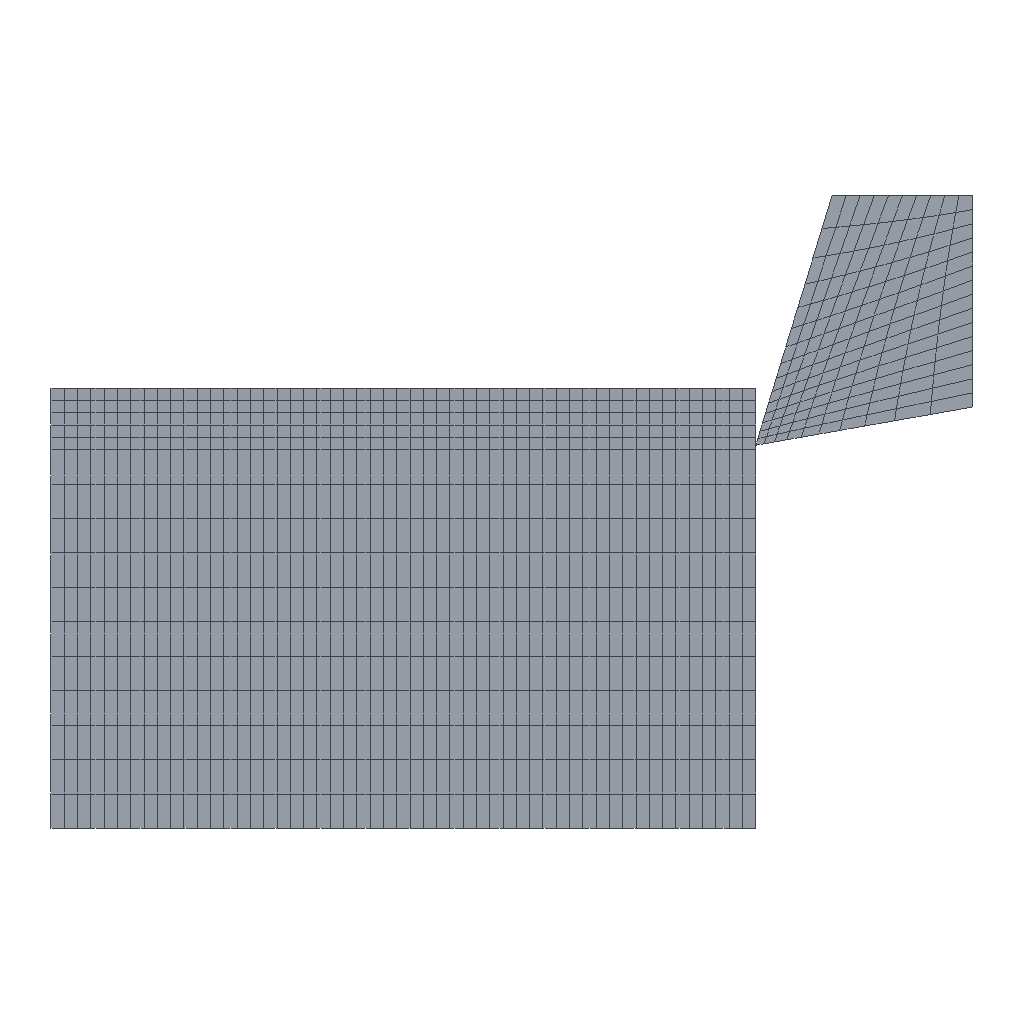Simulation study | abaqus
Set-up summary:
category,name,step,type,value,unit,region
solver,abaqus
solver,version,,,Abaqus/Explicit 2020
units,not stated in the deck,,not stated
analysis,deck,,dynamic temperature-displacement,dynamic temperature-displacement
load_step,Step-1,Step-1,dynamic temperature-displacement
load_step,requested,,,1
mesh,nodes,,,1094
mesh,elements,,,998
element_type,CPE4RT,,plane,998
load,load commands in deck,,count,1
bc,support commands in deck,,count,4
material,CFRP,,in results
material,CFRP-COPY,,in results
material,TOOL,,in results
check,setup vs results,,match,"per instance, exact: element labels, types and connectivity; labels of the nodes the elements use; coordinates of those nodes at SINGLE_PRECISION in 2 of 2 instance(s)"
Abaqus input file, long lists of numbers shortened:
*Heading
** Job name: Job-1 Model name: Model-1-Copy
** Generated by: Abaqus/CAE 2020
*Preprint, echo=NO, model=NO, history=NO, contact=NO
**
** PARTS
**
*Part, name=tool
*Node
      1,           0.,           0.
      2,  0.9701,  0.1711
** (174 more lines like these left out)
*Element, type=CPE4RT
  1,   1,   2,  13,  12
  2,   2,   3,  14,  13
** (148 more lines like these left out)
*Nset, nset=Set-1, generate
   1,  176,    1
*Elset, elset=Set-1, generate
   1,  150,    1
** Section: tool
*Solid Section, elset=Set-1, material=tool
,
*End Part
**
*Part, name=work
*Node
      1,          80.,          -7.
      2,           0.,          -7.
** (916 more lines like these left out)
*Element, type=CPE4RT
  1,   1,   7, 191, 130
  2,   7,   8, 192, 191
** (846 more lines like these left out)
*Nset, nset=Set-6, generate
   1,  918,    1
*Elset, elset=Set-6, generate
   1,  848,    1
*Nset, nset=Set-10
   1,   2,   5,   6,   7,   8,   9,  10,  11,  12,  13,  14,  15,  16,  17,  18
  19,  20,  21,  22,  23,  24,  25,  26,  27,  28,  29,  30,  31,  32,  33,  34
** (19 more lines like these left out)
*Elset, elset=Set-10, generate
 584,  848,    1
*Nset, nset=Set-11
   1,   2,   3,   4,   7,   8,   9,  10,  11,  12,  13,  14,  15,  16,  17,  18
  19,  20,  21,  22,  23,  24,  25,  26,  27,  28,  29,  30,  31,  32,  33,  34
** (39 more lines like these left out)
*Elset, elset=Set-11, generate
   1,  583,    1
*Nset, nset=Set-12, generate
   1,  918,    1
*Elset, elset=Set-12, generate
   1,  848,    1
*Orientation, name=Ori-1
1., 0., 0., 0., 1., 0.
3, 0.
** Section: work
*Solid Section, elset=Set-12, orientation=Ori-1, material=cfrp
,
*End Part
**
**
** ASSEMBLY
**
*Assembly, name=Assembly
**
*Instance, name=tool-1, part=tool
         80.,         -6.5,           0.
*End Instance
**
*Instance, name=work-1, part=work
*End Instance
**
*Node
      1,   104.667,    21.85,           0.
*Nset, nset=Set-1, instance=work-1
   3,   4,  69,  70,  71,  72,  73,  74,  75,  76,  77,  78,  79,  80,  81,  82
  83,  84,  85,  86,  87,  88,  89,  90,  91,  92,  93,  94,  95,  96,  97,  98
** (2 more lines like these left out)
*Elset, elset=Set-1, instance=work-1, generate
 531,  583,    1
*Nset, nset=Set-5
 1,
*Nset, nset=Set-6
 1,
*Nset, nset=Set-7, instance=work-1
   3,   4,  69,  70,  71,  72,  73,  74,  75,  76,  77,  78,  79,  80,  81,  82
  83,  84,  85,  86,  87,  88,  89,  90,  91,  92,  93,  94,  95,  96,  97,  98
** (2 more lines like these left out)
*Elset, elset=Set-7, instance=work-1, generate
 531,  583,    1
*Nset, nset=Set-9, instance=work-1
   2,   3,   4,  59,  60,  61,  62,  63,  64,  65,  66,  67,  68,  69,  70,  71
  72,  73,  74,  75,  76,  77,  78,  79,  80,  81,  82,  83,  84,  85,  86,  87
** (3 more lines like these left out)
*Elset, elset=Set-9, instance=work-1
  53, 106, 159, 212, 265, 318, 371, 424, 477, 530, 531, 532, 533, 534, 535, 536
 537, 538, 539, 540, 541, 542, 543, 544, 545, 546, 547, 548, 549, 550, 551, 552
** (2 more lines like these left out)
*Nset, nset=b_Set-2, instance=tool-1, generate
   1,  176,    1
*Elset, elset=b_Set-2, instance=tool-1, generate
   1,  150,    1
*Nset, nset=s_Set-4, instance=work-1
   5,   6, 135, 136, 137, 138, 139, 140, 141, 142, 143, 144, 145, 146, 147, 148
 149, 150, 151, 152, 153, 154, 155, 156, 157, 158, 159, 160, 161, 162, 163, 164
** (2 more lines like these left out)
*Elset, elset=s_Set-4, instance=work-1, generate
 796,  848,    1
*Nset, nset=s_Set-8, instance=work-1
   1,   2,   5,   6,   7,   8,   9,  10,  11,  12,  13,  14,  15,  16,  17,  18
  19,  20,  21,  22,  23,  24,  25,  26,  27,  28,  29,  30,  31,  32,  33,  34
** (19 more lines like these left out)
*Elset, elset=s_Set-8, instance=work-1, generate
 584,  848,    1
*Nset, nset=_PickedSet9, internal
 1,
*Elset, elset=_m_Surf-1_S1, internal, instance=tool-1, generate
  1,  10,   1
*Elset, elset=_m_Surf-1_S4, internal, instance=tool-1, generate
   1,  141,   10
*Surface, type=ELEMENT, name=m_Surf-1
_m_Surf-1_S1, S1
_m_Surf-1_S4, S4
*Surface, type=NODE, name=s_Set-8_CNS_, internal
s_Set-8, 1.
** Constraint: Constraint-1
*Rigid Body, ref node=_PickedSet9, elset=b_Set-2
*End Assembly
*Amplitude, name=Amp-1
             0.,              0.,              1.,              1.
**
** MATERIALS
**
*Material, name=cfrp
*Conductivity
 0.5,
*Damage Initiation, criterion=SHEAR
 0.7,0.,0.
*Damage Evolution, type=DISPLACEMENT
 0.01,
*Density
 2e-09,
*Elastic
56000., 0.3
*Expansion
 8.5e-06,
*Plastic
250.,   0.
300., 0.05
350.,  0.1
*Specific Heat
 8e+08,
*Material, name=cfrp-Copy
*Conductivity
 0.5,
*Density
 2e-09,
*Elastic
56000., 0.3
*Expansion
 8.5e-06,
*Plastic
250.,   0.
300., 0.05
350.,  0.1
*Specific Heat
 8e+08,
*Material, name=tool
*Conductivity
45.,
*Density
 7.8e-09,
*Elastic
210000., 0.3
*Specific Heat
 4.6e+08,
**
** INTERACTION PROPERTIES
**
*Surface Interaction, name=IntProp-1
*Friction
 0.3,
*Surface Behavior, pressure-overclosure=HARD
*Gap Conductance
 0.0001,   0.
     0., 0.01
** ----------------------------------------------------------------
**
** STEP: Step-1
**
*Step, name=Step-1, nlgeom=YES
*Dynamic Temperature-displacement, Explicit
, 1.
*Bulk Viscosity
0.06, 1.2
** Mass Scaling: Semi-Automatic
**               Whole Model
*Fixed Mass Scaling, factor=50.
**
** BOUNDARY CONDITIONS
**
** Name: BC-1 Type: 对称/反对称/完全固定
*Boundary
Set-9, ENCASTRE
** Name: [REDACTED] : Displacement/rotation angle
*Boundary, amplitude=Amp-1
Set-6, 1, 1, -80.
Set-6, 2, 2
Set-6, 6, 6
**
** INTERACTIONS
**
** Interaction: Int-1
*Contact Pair, interaction=IntProp-1, mechanical constraint=KINEMATIC, cpset=Int-1
m_Surf-1, s_Set-8_CNS_
** Interaction: Int-2
*Contact, op=NEW
*Contact Inclusions, ALL EXTERIOR
*Contact Property Assignment
 ,  , IntProp-1
**
** OUTPUT REQUESTS
**
*Restart, write, number interval=1, time marks=NO
**
** FIELD OUTPUT: F-Output-1
**
*Output, field, number interval=50
*Node Output
CF, NT, RF, RM, RT, U, V
*Element Output, directions=YES
DAMAGEC, DAMAGET, E, LE, MISES, MISESMAX, PE, PEEQ, PEEQMAX, PEEQT, S, SDEG, SF, STATUS, TEMP, YIELDPOT
*Contact Output
CDISP, CSTRESS
**
** HISTORY OUTPUT: H-Output-1
**
*Output, history, time interval=2e-05
*Node Output, nset=Set-5
RF1, RF2
*End Step
Results summary:
result,step,Step-1,partial,increments=642947 time=0.58/1.0
result,analysis,,,"dynamic temperature-displacement, explict"
result,last_loadstep,,,1
result,primary field,,,"U, NT11"
result,reaction total,,FX,-26.558,model units
result,reaction total,,FY,14.675,model units
result,reaction total,,FZ,0.0,model units